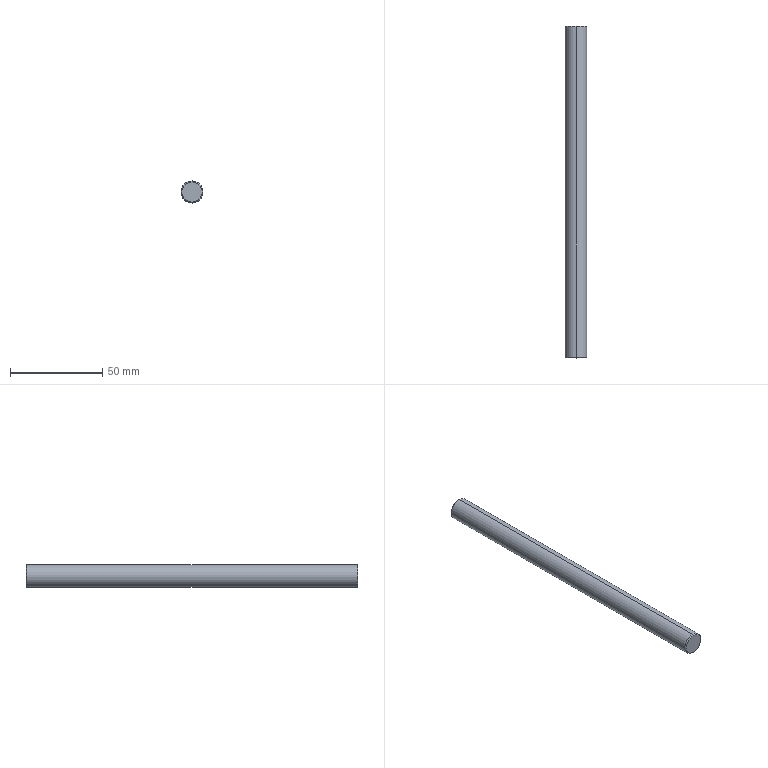Part | STEP file | ND25021-01-JDKM-21-GJ | 1 solid | 8 faces | box 12 x 180 x 12 mm | volume 20348 mm3 | cone 4 | cylinder 2 | plane 2 | commonest cylinder face diameters 12 x2
STEP:
#1=CARTESIAN_POINT('',(0.,0.,0.));
#2=DIRECTION('',(0.,0.,1.));
#3=DIRECTION('',(1.,0.,0.));
#4=AXIS2_PLACEMENT_3D('',#1,#2,#3);
#5=CARTESIAN_POINT('',(0.,180.,5.5));
#6=VERTEX_POINT('',#5);
#7=CARTESIAN_POINT('',(0.,180.,-5.5));
#8=VERTEX_POINT('',#7);
#9=CARTESIAN_POINT('',(0.,180.,0.));
#10=DIRECTION('',(0.,1.,0.));
#11=DIRECTION('',(0.,0.,1.));
#12=AXIS2_PLACEMENT_3D('',#9,#10,#11);
#13=CIRCLE('',#12,5.5);
#14=CARTESIAN_POINT('',(0.,180.,0.));
#15=DIRECTION('',(0.,-1.,0.));
#16=DIRECTION('',(0.,0.,-1.));
#17=AXIS2_PLACEMENT_3D('',#14,#15,#16);
#18=CONICAL_SURFACE('',#17,5.5,0.7854);
#19=CARTESIAN_POINT('',(3.142,0.));
#20=DIRECTION('',(-1.,0.));
#21=VECTOR('',#20,1.);
#22=LINE('',#19,#21);
#23=(GEOMETRIC_REPRESENTATION_CONTEXT(2)PARAMETRIC_REPRESENTATION_CONTEXT()REPRESENTATION_CONTEXT('',''));
#24=DEFINITIONAL_REPRESENTATION('',(#22),#23);
#25=PCURVE('',#18,#24);
#26=CARTESIAN_POINT('',(0.,180.,0.));
#27=DIRECTION('',(0.,1.,0.));
#28=DIRECTION('',(0.,0.,1.));
#29=AXIS2_PLACEMENT_3D('',#26,#27,#28);
#30=PLANE('',#29);
#31=CARTESIAN_POINT('',(0.,0.));
#32=DIRECTION('',(1.,0.));
#33=AXIS2_PLACEMENT_2D('',#31,#32);
#34=CIRCLE('',#33,5.5);
#35=(GEOMETRIC_REPRESENTATION_CONTEXT(2)PARAMETRIC_REPRESENTATION_CONTEXT()REPRESENTATION_CONTEXT('',''));
#36=DEFINITIONAL_REPRESENTATION('',(#34),#35);
#37=PCURVE('',#30,#36);
#38=SURFACE_CURVE('',#13,(#25,#37),.PCURVE_S1.);
#39=EDGE_CURVE('',#6,#8,#38,.T.);
#40=ORIENTED_EDGE('',*,*,#39,.F.);
#41=CARTESIAN_POINT('',(0.,179.5,6.));
#42=VERTEX_POINT('',#41);
#43=CARTESIAN_POINT('',(0.,180.,5.5));
#44=DIRECTION('',(0.,-0.7071,0.7071));
#45=VECTOR('',#44,1.);
#46=LINE('',#43,#45);
#47=CARTESIAN_POINT('',(3.142,0.));
#48=DIRECTION('',(0.,1.));
#49=VECTOR('',#48,1.);
#50=LINE('',#47,#49);
#51=(GEOMETRIC_REPRESENTATION_CONTEXT(2)PARAMETRIC_REPRESENTATION_CONTEXT()REPRESENTATION_CONTEXT('',''));
#52=DEFINITIONAL_REPRESENTATION('',(#50),#51);
#53=PCURVE('',#18,#52);
#54=CARTESIAN_POINT('',(0.,180.,0.));
#55=DIRECTION('',(0.,-1.,0.));
#56=DIRECTION('',(0.,0.,-1.));
#57=AXIS2_PLACEMENT_3D('',#54,#55,#56);
#58=CONICAL_SURFACE('',#57,5.5,0.7854);
#59=CARTESIAN_POINT('',(3.142,0.));
#60=DIRECTION('',(0.,1.));
#61=VECTOR('',#60,1.);
#62=LINE('',#59,#61);
#63=(GEOMETRIC_REPRESENTATION_CONTEXT(2)PARAMETRIC_REPRESENTATION_CONTEXT()REPRESENTATION_CONTEXT('',''));
#64=DEFINITIONAL_REPRESENTATION('',(#62),#63);
#65=PCURVE('',#58,#64);
#66=SURFACE_CURVE('',#46,(#53,#65),.PCURVE_S1.);
#67=EDGE_CURVE('',#6,#42,#66,.T.);
#68=ORIENTED_EDGE('',*,*,#67,.T.);
#69=CARTESIAN_POINT('',(0.,179.5,-6.));
#70=VERTEX_POINT('',#69);
#71=CARTESIAN_POINT('',(0.,179.5,0.));
#72=DIRECTION('',(0.,-1.,0.));
#73=DIRECTION('',(0.,0.,1.));
#74=AXIS2_PLACEMENT_3D('',#71,#72,#73);
#75=CIRCLE('',#74,6.);
#76=CARTESIAN_POINT('',(-3.142,0.5));
#77=DIRECTION('',(1.,0.));
#78=VECTOR('',#77,1.);
#79=LINE('',#76,#78);
#80=(GEOMETRIC_REPRESENTATION_CONTEXT(2)PARAMETRIC_REPRESENTATION_CONTEXT()REPRESENTATION_CONTEXT('',''));
#81=DEFINITIONAL_REPRESENTATION('',(#79),#80);
#82=PCURVE('',#18,#81);
#83=CARTESIAN_POINT('',(0.,180.,0.));
#84=DIRECTION('',(0.,-1.,0.));
#85=DIRECTION('',(0.,0.,-1.));
#86=AXIS2_PLACEMENT_3D('',#83,#84,#85);
#87=CYLINDRICAL_SURFACE('',#86,6.);
#88=CARTESIAN_POINT('',(-3.142,0.5));
#89=DIRECTION('',(1.,0.));
#90=VECTOR('',#89,1.);
#91=LINE('',#88,#90);
#92=(GEOMETRIC_REPRESENTATION_CONTEXT(2)PARAMETRIC_REPRESENTATION_CONTEXT()REPRESENTATION_CONTEXT('',''));
#93=DEFINITIONAL_REPRESENTATION('',(#91),#92);
#94=PCURVE('',#87,#93);
#95=SURFACE_CURVE('',#75,(#82,#94),.PCURVE_S1.);
#96=EDGE_CURVE('',#70,#42,#95,.T.);
#97=ORIENTED_EDGE('',*,*,#96,.F.);
#98=CARTESIAN_POINT('',(0.,180.,-5.5));
#99=DIRECTION('',(0.,-0.7071,-0.7071));
#100=VECTOR('',#99,1.);
#101=LINE('',#98,#100);
#102=CARTESIAN_POINT('',(0.,0.));
#103=DIRECTION('',(0.,1.));
#104=VECTOR('',#103,1.);
#105=LINE('',#102,#104);
#106=(GEOMETRIC_REPRESENTATION_CONTEXT(2)PARAMETRIC_REPRESENTATION_CONTEXT()REPRESENTATION_CONTEXT('',''));
#107=DEFINITIONAL_REPRESENTATION('',(#105),#106);
#108=PCURVE('',#18,#107);
#109=CARTESIAN_POINT('',(6.283,0.));
#110=DIRECTION('',(0.,1.));
#111=VECTOR('',#110,1.);
#112=LINE('',#109,#111);
#113=(GEOMETRIC_REPRESENTATION_CONTEXT(2)PARAMETRIC_REPRESENTATION_CONTEXT()REPRESENTATION_CONTEXT('',''));
#114=DEFINITIONAL_REPRESENTATION('',(#112),#113);
#115=PCURVE('',#58,#114);
#116=SURFACE_CURVE('',#101,(#108,#115),.PCURVE_S1.);
#117=EDGE_CURVE('',#8,#70,#116,.T.);
#118=ORIENTED_EDGE('',*,*,#117,.F.);
#119=EDGE_LOOP('',(#40,#68,#97,#118));
#120=FACE_BOUND('',#119,.T.);
#121=ADVANCED_FACE('',(#120),#18,.T.);
#122=CARTESIAN_POINT('',(0.,0.,-5.5));
#123=VERTEX_POINT('',#122);
#124=CARTESIAN_POINT('',(0.,0.,5.5));
#125=VERTEX_POINT('',#124);
#126=CARTESIAN_POINT('',(0.,0.,0.));
#127=DIRECTION('',(0.,-1.,0.));
#128=DIRECTION('',(0.,0.,1.));
#129=AXIS2_PLACEMENT_3D('',#126,#127,#128);
#130=CIRCLE('',#129,5.5);
#131=CARTESIAN_POINT('',(0.,0.5,0.));
#132=DIRECTION('',(0.,1.,0.));
#133=DIRECTION('',(0.,0.,1.));
#134=AXIS2_PLACEMENT_3D('',#131,#132,#133);
#135=CONICAL_SURFACE('',#134,6.,0.7854);
#136=CARTESIAN_POINT('',(6.283,-0.5));
#137=DIRECTION('',(-1.,0.));
#138=VECTOR('',#137,1.);
#139=LINE('',#136,#138);
#140=(GEOMETRIC_REPRESENTATION_CONTEXT(2)PARAMETRIC_REPRESENTATION_CONTEXT()REPRESENTATION_CONTEXT('',''));
#141=DEFINITIONAL_REPRESENTATION('',(#139),#140);
#142=PCURVE('',#135,#141);
#143=CARTESIAN_POINT('',(0.,0.,0.));
#144=DIRECTION('',(0.,1.,0.));
#145=DIRECTION('',(0.,0.,1.));
#146=AXIS2_PLACEMENT_3D('',#143,#144,#145);
#147=PLANE('',#146);
#148=CARTESIAN_POINT('',(5.5,0.));
#149=CARTESIAN_POINT('',(5.5,-9.526));
#150=CARTESIAN_POINT('',(-2.75,-4.763));
#151=CARTESIAN_POINT('',(-11.,0.));
#152=CARTESIAN_POINT('',(-2.75,4.763));
#153=CARTESIAN_POINT('',(5.5,9.526));
#154=CARTESIAN_POINT('',(5.5,0.));
#155=(BOUNDED_CURVE()B_SPLINE_CURVE(2,(#148,#149,#150,#151,#152,#153,#154),.UNSPECIFIED.,.T.,.F.)B_SPLINE_CURVE_WITH_KNOTS((1,2,2,2,2,1),(-2.094,0.,2.094,4.189,6.283,8.378),.UNSPECIFIED.)CURVE()GEOMETRIC_REPRESENTATION_ITEM()RATIONAL_B_SPLINE_CURVE((1.,0.5,1.,0.5,1.,0.5,1.))REPRESENTATION_ITEM(''));
#156=(GEOMETRIC_REPRESENTATION_CONTEXT(2)PARAMETRIC_REPRESENTATION_CONTEXT()REPRESENTATION_CONTEXT('',''));
#157=DEFINITIONAL_REPRESENTATION('',(#155),#156);
#158=PCURVE('',#147,#157);
#159=SURFACE_CURVE('',#130,(#142,#158),.PCURVE_S1.);
#160=EDGE_CURVE('',#123,#125,#159,.T.);
#161=ORIENTED_EDGE('',*,*,#160,.F.);
#162=CARTESIAN_POINT('',(0.,0.5,-6.));
#163=VERTEX_POINT('',#162);
#164=CARTESIAN_POINT('',(0.,0.5,-6.));
#165=DIRECTION('',(0.,0.7071,-0.7071));
#166=VECTOR('',#165,1.);
#167=LINE('',#164,#166);
#168=CARTESIAN_POINT('',(3.142,0.));
#169=DIRECTION('',(0.,1.));
#170=VECTOR('',#169,1.);
#171=LINE('',#168,#170);
#172=(GEOMETRIC_REPRESENTATION_CONTEXT(2)PARAMETRIC_REPRESENTATION_CONTEXT()REPRESENTATION_CONTEXT('',''));
#173=DEFINITIONAL_REPRESENTATION('',(#171),#172);
#174=PCURVE('',#135,#173);
#175=CARTESIAN_POINT('',(0.,0.5,0.));
#176=DIRECTION('',(0.,1.,0.));
#177=DIRECTION('',(0.,0.,1.));
#178=AXIS2_PLACEMENT_3D('',#175,#176,#177);
#179=CONICAL_SURFACE('',#178,6.,0.7854);
#180=CARTESIAN_POINT('',(3.142,0.));
#181=DIRECTION('',(0.,1.));
#182=VECTOR('',#181,1.);
#183=LINE('',#180,#182);
#184=(GEOMETRIC_REPRESENTATION_CONTEXT(2)PARAMETRIC_REPRESENTATION_CONTEXT()REPRESENTATION_CONTEXT('',''));
#185=DEFINITIONAL_REPRESENTATION('',(#183),#184);
#186=PCURVE('',#179,#185);
#187=SURFACE_CURVE('',#167,(#174,#186),.PCURVE_S1.);
#188=EDGE_CURVE('',#123,#163,#187,.T.);
#189=ORIENTED_EDGE('',*,*,#188,.T.);
#190=CARTESIAN_POINT('',(0.,0.5,6.));
#191=VERTEX_POINT('',#190);
#192=CARTESIAN_POINT('',(0.,0.5,0.));
#193=DIRECTION('',(0.,1.,0.));
#194=DIRECTION('',(0.,0.,1.));
#195=AXIS2_PLACEMENT_3D('',#192,#193,#194);
#196=CIRCLE('',#195,6.);
#197=CARTESIAN_POINT('',(0.,0.));
#198=DIRECTION('',(1.,0.));
#199=VECTOR('',#198,1.);
#200=LINE('',#197,#199);
#201=(GEOMETRIC_REPRESENTATION_CONTEXT(2)PARAMETRIC_REPRESENTATION_CONTEXT()REPRESENTATION_CONTEXT('',''));
#202=DEFINITIONAL_REPRESENTATION('',(#200),#201);
#203=PCURVE('',#135,#202);
#204=CARTESIAN_POINT('',(3.142,179.5));
#205=DIRECTION('',(-1.,0.));
#206=VECTOR('',#205,1.);
#207=LINE('',#204,#206);
#208=(GEOMETRIC_REPRESENTATION_CONTEXT(2)PARAMETRIC_REPRESENTATION_CONTEXT()REPRESENTATION_CONTEXT('',''));
#209=DEFINITIONAL_REPRESENTATION('',(#207),#208);
#210=PCURVE('',#87,#209);
#211=SURFACE_CURVE('',#196,(#203,#210),.PCURVE_S1.);
#212=EDGE_CURVE('',#191,#163,#211,.T.);
#213=ORIENTED_EDGE('',*,*,#212,.F.);
#214=CARTESIAN_POINT('',(0.,0.5,6.));
#215=DIRECTION('',(0.,0.7071,0.7071));
#216=VECTOR('',#215,1.);
#217=LINE('',#214,#216);
#218=CARTESIAN_POINT('',(0.,0.));
#219=DIRECTION('',(0.,1.));
#220=VECTOR('',#219,1.);
#221=LINE('',#218,#220);
#222=(GEOMETRIC_REPRESENTATION_CONTEXT(2)PARAMETRIC_REPRESENTATION_CONTEXT()REPRESENTATION_CONTEXT('',''));
#223=DEFINITIONAL_REPRESENTATION('',(#221),#222);
#224=PCURVE('',#135,#223);
#225=CARTESIAN_POINT('',(6.283,0.));
#226=DIRECTION('',(0.,1.));
#227=VECTOR('',#226,1.);
#228=LINE('',#225,#227);
#229=(GEOMETRIC_REPRESENTATION_CONTEXT(2)PARAMETRIC_REPRESENTATION_CONTEXT()REPRESENTATION_CONTEXT('',''));
#230=DEFINITIONAL_REPRESENTATION('',(#228),#229);
#231=PCURVE('',#179,#230);
#232=SURFACE_CURVE('',#217,(#224,#231),.PCURVE_S1.);
#233=EDGE_CURVE('',#125,#191,#232,.T.);
#234=ORIENTED_EDGE('',*,*,#233,.F.);
#235=EDGE_LOOP('',(#161,#189,#213,#234));
#236=FACE_BOUND('',#235,.T.);
#237=ADVANCED_FACE('',(#236),#135,.T.);
#238=ORIENTED_EDGE('',*,*,#96,.T.);
#239=CARTESIAN_POINT('',(0.,180.,6.));
#240=DIRECTION('',(0.,-1.,0.));
#241=VECTOR('',#240,1.);
#242=LINE('',#239,#241);
#243=CARTESIAN_POINT('',(3.142,0.));
#244=DIRECTION('',(0.,1.));
#245=VECTOR('',#244,1.);
#246=LINE('',#243,#245);
#247=(GEOMETRIC_REPRESENTATION_CONTEXT(2)PARAMETRIC_REPRESENTATION_CONTEXT()REPRESENTATION_CONTEXT('',''));
#248=DEFINITIONAL_REPRESENTATION('',(#246),#247);
#249=PCURVE('',#87,#248);
#250=CARTESIAN_POINT('',(0.,180.,0.));
#251=DIRECTION('',(0.,-1.,0.));
#252=DIRECTION('',(0.,0.,-1.));
#253=AXIS2_PLACEMENT_3D('',#250,#251,#252);
#254=CYLINDRICAL_SURFACE('',#253,6.);
#255=CARTESIAN_POINT('',(3.142,0.));
#256=DIRECTION('',(0.,1.));
#257=VECTOR('',#256,1.);
#258=LINE('',#255,#257);
#259=(GEOMETRIC_REPRESENTATION_CONTEXT(2)PARAMETRIC_REPRESENTATION_CONTEXT()REPRESENTATION_CONTEXT('',''));
#260=DEFINITIONAL_REPRESENTATION('',(#258),#259);
#261=PCURVE('',#254,#260);
#262=SURFACE_CURVE('',#242,(#249,#261),.PCURVE_S1.);
#263=EDGE_CURVE('',#42,#191,#262,.T.);
#264=ORIENTED_EDGE('',*,*,#263,.T.);
#265=ORIENTED_EDGE('',*,*,#212,.T.);
#266=CARTESIAN_POINT('',(0.,180.,-6.));
#267=DIRECTION('',(0.,-1.,0.));
#268=VECTOR('',#267,1.);
#269=LINE('',#266,#268);
#270=CARTESIAN_POINT('',(0.,0.));
#271=DIRECTION('',(0.,1.));
#272=VECTOR('',#271,1.);
#273=LINE('',#270,#272);
#274=(GEOMETRIC_REPRESENTATION_CONTEXT(2)PARAMETRIC_REPRESENTATION_CONTEXT()REPRESENTATION_CONTEXT('',''));
#275=DEFINITIONAL_REPRESENTATION('',(#273),#274);
#276=PCURVE('',#87,#275);
#277=CARTESIAN_POINT('',(6.283,0.));
#278=DIRECTION('',(0.,1.));
#279=VECTOR('',#278,1.);
#280=LINE('',#277,#279);
#281=(GEOMETRIC_REPRESENTATION_CONTEXT(2)PARAMETRIC_REPRESENTATION_CONTEXT()REPRESENTATION_CONTEXT('',''));
#282=DEFINITIONAL_REPRESENTATION('',(#280),#281);
#283=PCURVE('',#254,#282);
#284=SURFACE_CURVE('',#269,(#276,#283),.PCURVE_S1.);
#285=EDGE_CURVE('',#70,#163,#284,.T.);
#286=ORIENTED_EDGE('',*,*,#285,.F.);
#287=EDGE_LOOP('',(#238,#264,#265,#286));
#288=FACE_BOUND('',#287,.T.);
#289=ADVANCED_FACE('',(#288),#87,.T.);
#290=ORIENTED_EDGE('',*,*,#263,.F.);
#291=CARTESIAN_POINT('',(0.,179.5,0.));
#292=DIRECTION('',(0.,-1.,0.));
#293=DIRECTION('',(0.,0.,1.));
#294=AXIS2_PLACEMENT_3D('',#291,#292,#293);
#295=CIRCLE('',#294,6.);
#296=CARTESIAN_POINT('',(3.142,0.5));
#297=DIRECTION('',(1.,0.));
#298=VECTOR('',#297,1.);
#299=LINE('',#296,#298);
#300=(GEOMETRIC_REPRESENTATION_CONTEXT(2)PARAMETRIC_REPRESENTATION_CONTEXT()REPRESENTATION_CONTEXT('',''));
#301=DEFINITIONAL_REPRESENTATION('',(#299),#300);
#302=PCURVE('',#254,#301);
#303=CARTESIAN_POINT('',(3.142,0.5));
#304=DIRECTION('',(1.,0.));
#305=VECTOR('',#304,1.);
#306=LINE('',#303,#305);
#307=(GEOMETRIC_REPRESENTATION_CONTEXT(2)PARAMETRIC_REPRESENTATION_CONTEXT()REPRESENTATION_CONTEXT('',''));
#308=DEFINITIONAL_REPRESENTATION('',(#306),#307);
#309=PCURVE('',#58,#308);
#310=SURFACE_CURVE('',#295,(#302,#309),.PCURVE_S1.);
#311=EDGE_CURVE('',#42,#70,#310,.T.);
#312=ORIENTED_EDGE('',*,*,#311,.T.);
#313=ORIENTED_EDGE('',*,*,#285,.T.);
#314=CARTESIAN_POINT('',(0.,0.5,0.));
#315=DIRECTION('',(0.,1.,0.));
#316=DIRECTION('',(0.,0.,1.));
#317=AXIS2_PLACEMENT_3D('',#314,#315,#316);
#318=CIRCLE('',#317,6.);
#319=CARTESIAN_POINT('',(9.425,179.5));
#320=DIRECTION('',(-1.,0.));
#321=VECTOR('',#320,1.);
#322=LINE('',#319,#321);
#323=(GEOMETRIC_REPRESENTATION_CONTEXT(2)PARAMETRIC_REPRESENTATION_CONTEXT()REPRESENTATION_CONTEXT('',''));
#324=DEFINITIONAL_REPRESENTATION('',(#322),#323);
#325=PCURVE('',#254,#324);
#326=CARTESIAN_POINT('',(0.,0.));
#327=DIRECTION('',(1.,0.));
#328=VECTOR('',#327,1.);
#329=LINE('',#326,#328);
#330=(GEOMETRIC_REPRESENTATION_CONTEXT(2)PARAMETRIC_REPRESENTATION_CONTEXT()REPRESENTATION_CONTEXT('',''));
#331=DEFINITIONAL_REPRESENTATION('',(#329),#330);
#332=PCURVE('',#179,#331);
#333=SURFACE_CURVE('',#318,(#325,#332),.PCURVE_S1.);
#334=EDGE_CURVE('',#163,#191,#333,.T.);
#335=ORIENTED_EDGE('',*,*,#334,.T.);
#336=EDGE_LOOP('',(#290,#312,#313,#335));
#337=FACE_BOUND('',#336,.T.);
#338=ADVANCED_FACE('',(#337),#254,.T.);
#339=CARTESIAN_POINT('',(0.,180.,0.));
#340=DIRECTION('',(0.,1.,0.));
#341=DIRECTION('',(0.,0.,1.));
#342=AXIS2_PLACEMENT_3D('',#339,#340,#341);
#343=CIRCLE('',#342,5.5);
#344=CARTESIAN_POINT('',(0.,0.));
#345=DIRECTION('',(1.,0.));
#346=AXIS2_PLACEMENT_2D('',#344,#345);
#347=CIRCLE('',#346,5.5);
#348=(GEOMETRIC_REPRESENTATION_CONTEXT(2)PARAMETRIC_REPRESENTATION_CONTEXT()REPRESENTATION_CONTEXT('',''));
#349=DEFINITIONAL_REPRESENTATION('',(#347),#348);
#350=PCURVE('',#30,#349);
#351=CARTESIAN_POINT('',(9.425,0.));
#352=DIRECTION('',(-1.,0.));
#353=VECTOR('',#352,1.);
#354=LINE('',#351,#353);
#355=(GEOMETRIC_REPRESENTATION_CONTEXT(2)PARAMETRIC_REPRESENTATION_CONTEXT()REPRESENTATION_CONTEXT('',''));
#356=DEFINITIONAL_REPRESENTATION('',(#354),#355);
#357=PCURVE('',#58,#356);
#358=SURFACE_CURVE('',#343,(#350,#357),.PCURVE_S1.);
#359=EDGE_CURVE('',#8,#6,#358,.T.);
#360=ORIENTED_EDGE('',*,*,#359,.T.);
#361=ORIENTED_EDGE('',*,*,#39,.T.);
#362=EDGE_LOOP('',(#360,#361));
#363=FACE_BOUND('',#362,.T.);
#364=ADVANCED_FACE('',(#363),#30,.T.);
#365=CARTESIAN_POINT('',(0.,0.,0.));
#366=DIRECTION('',(0.,-1.,0.));
#367=DIRECTION('',(0.,0.,1.));
#368=AXIS2_PLACEMENT_3D('',#365,#366,#367);
#369=CIRCLE('',#368,5.5);
#370=CARTESIAN_POINT('',(5.5,0.));
#371=CARTESIAN_POINT('',(5.5,-9.526));
#372=CARTESIAN_POINT('',(-2.75,-4.763));
#373=CARTESIAN_POINT('',(-11.,0.));
#374=CARTESIAN_POINT('',(-2.75,4.763));
#375=CARTESIAN_POINT('',(5.5,9.526));
#376=CARTESIAN_POINT('',(5.5,0.));
#377=(BOUNDED_CURVE()B_SPLINE_CURVE(2,(#370,#371,#372,#373,#374,#375,#376),.UNSPECIFIED.,.T.,.F.)B_SPLINE_CURVE_WITH_KNOTS((1,2,2,2,2,1),(-2.094,0.,2.094,4.189,6.283,8.378),.UNSPECIFIED.)CURVE()GEOMETRIC_REPRESENTATION_ITEM()RATIONAL_B_SPLINE_CURVE((1.,0.5,1.,0.5,1.,0.5,1.))REPRESENTATION_ITEM(''));
#378=(GEOMETRIC_REPRESENTATION_CONTEXT(2)PARAMETRIC_REPRESENTATION_CONTEXT()REPRESENTATION_CONTEXT('',''));
#379=DEFINITIONAL_REPRESENTATION('',(#377),#378);
#380=PCURVE('',#147,#379);
#381=CARTESIAN_POINT('',(6.283,-0.5));
#382=DIRECTION('',(-1.,0.));
#383=VECTOR('',#382,1.);
#384=LINE('',#381,#383);
#385=(GEOMETRIC_REPRESENTATION_CONTEXT(2)PARAMETRIC_REPRESENTATION_CONTEXT()REPRESENTATION_CONTEXT('',''));
#386=DEFINITIONAL_REPRESENTATION('',(#384),#385);
#387=PCURVE('',#179,#386);
#388=SURFACE_CURVE('',#369,(#380,#387),.PCURVE_S1.);
#389=EDGE_CURVE('',#125,#123,#388,.T.);
#390=ORIENTED_EDGE('',*,*,#389,.T.);
#391=ORIENTED_EDGE('',*,*,#160,.T.);
#392=EDGE_LOOP('',(#390,#391));
#393=FACE_BOUND('',#392,.T.);
#394=ADVANCED_FACE('',(#393),#147,.F.);
#395=ORIENTED_EDGE('',*,*,#188,.F.);
#396=ORIENTED_EDGE('',*,*,#389,.F.);
#397=ORIENTED_EDGE('',*,*,#233,.T.);
#398=ORIENTED_EDGE('',*,*,#334,.F.);
#399=EDGE_LOOP('',(#395,#396,#397,#398));
#400=FACE_BOUND('',#399,.T.);
#401=ADVANCED_FACE('',(#400),#179,.T.);
#402=ORIENTED_EDGE('',*,*,#67,.F.);
#403=ORIENTED_EDGE('',*,*,#359,.F.);
#404=ORIENTED_EDGE('',*,*,#117,.T.);
#405=ORIENTED_EDGE('',*,*,#311,.F.);
#406=EDGE_LOOP('',(#402,#403,#404,#405));
#407=FACE_BOUND('',#406,.T.);
#408=ADVANCED_FACE('',(#407),#58,.T.);
#409=CLOSED_SHELL('',(#121,#237,#289,#338,#364,#394,#401,#408));
#410=MANIFOLD_SOLID_BREP('',#409);
#411=(LENGTH_UNIT()NAMED_UNIT(*)SI_UNIT(.MILLI.,.METRE.));
#412=UNCERTAINTY_MEASURE_WITH_UNIT(LENGTH_MEASURE(0.0000001),#411,'','');
#413=(NAMED_UNIT(*)PLANE_ANGLE_UNIT()SI_UNIT($,.RADIAN.));
#414=(NAMED_UNIT(*)SI_UNIT($,.STERADIAN.)SOLID_ANGLE_UNIT());
#415=(GEOMETRIC_REPRESENTATION_CONTEXT(3)GLOBAL_UNCERTAINTY_ASSIGNED_CONTEXT((#412))GLOBAL_UNIT_ASSIGNED_CONTEXT((#411,#413,#414))REPRESENTATION_CONTEXT('',''));
#416=ADVANCED_BREP_SHAPE_REPRESENTATION('',(#4,#410),#415);